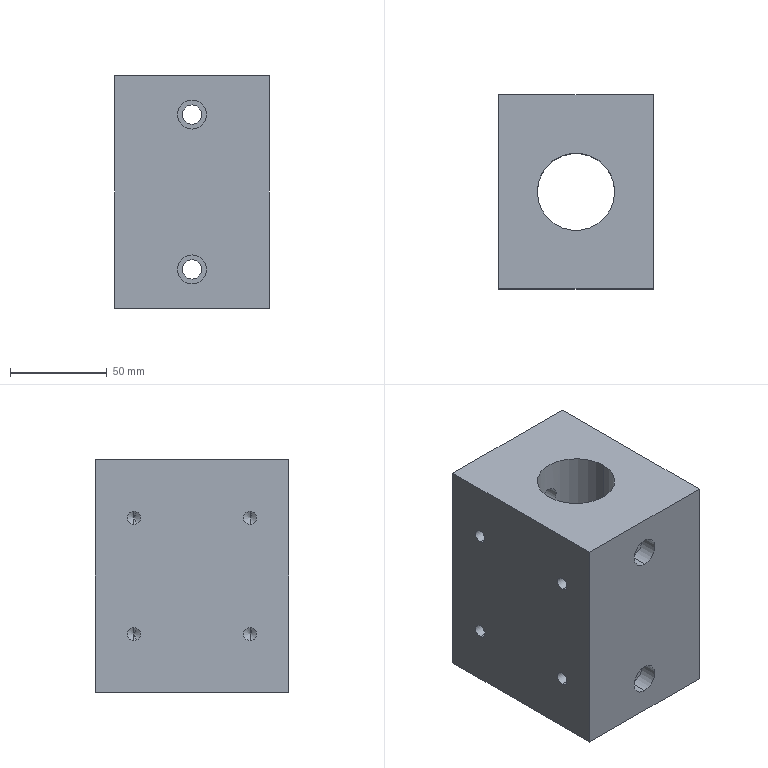Part | SolidWorks | features HoleWzd 5, ICE 4, Extrusion 1 | 1 solid | 62 faces | box 80 x 100 x 120 mm | volume 786189 mm3 | cylinder 36 | cone 16 | plane 10 | commonest cylinder face diameters 6.8 x18 10 x8 15 x8 40 x2